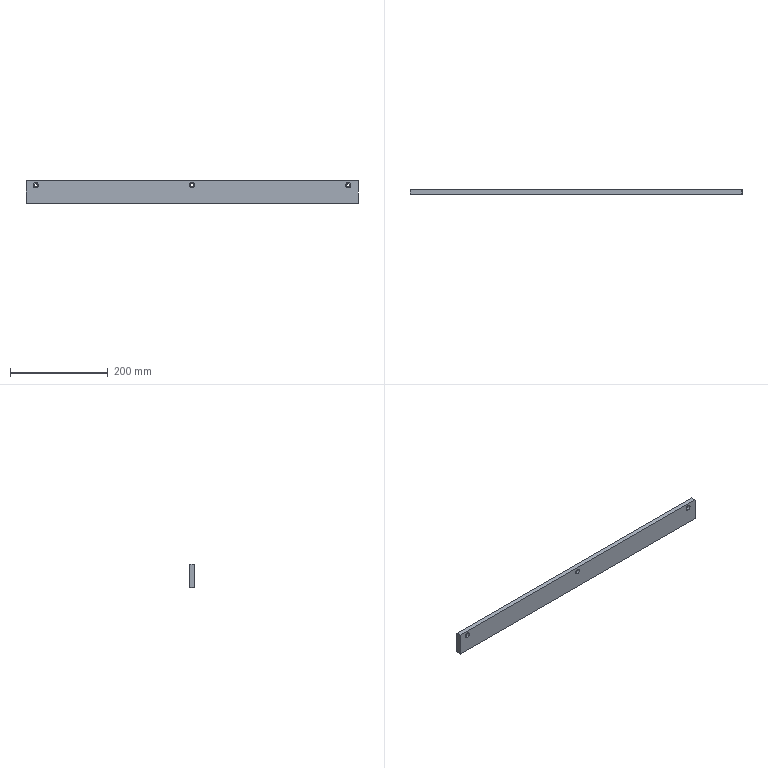Part | SolidWorks | features HoleWzd 2, Chamfer 1, Extrusion 1 | 1 solid | 157 faces | box 680 x 10 x 47.5 mm | volume 316323 mm3 | cylinder 78 | cone 66 | plane 13 | commonest cylinder face diameters 4.1 x66 6.6 x6 11 x6